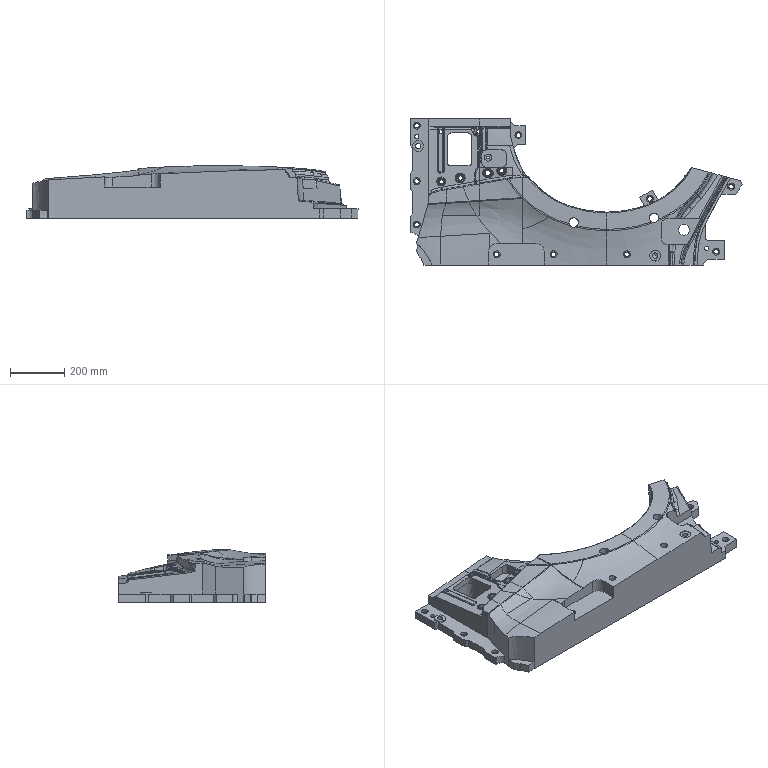Part | NX | features solid 2 | 1 solid | 529 faces | box 1225 x 540.01 x 193.375 mm | volume 39527545 mm3 | spline 329 | plane 128 | cylinder 70 | cone 1 | sphere 1 | commonest cylinder face diameters 17 x10 20 x9 25.5 x7 16 x6 40 x5 30 x4